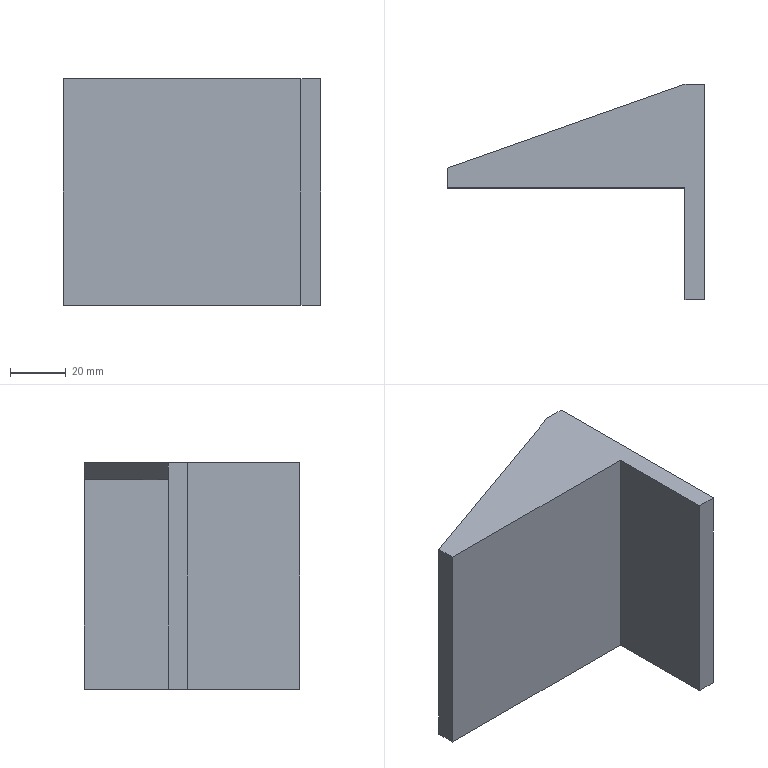Part | STEP file | Guide wheel mechanism revised.sldasm-Part-64 | 1 solid | 12 faces | box 92 x 77 x 81 mm | volume 99504 mm3 | plane 12
STEP:
#1=CARTESIAN_POINT('',(-42.5,0.,-40.5));
#2=VERTEX_POINT('',#1);
#3=CARTESIAN_POINT('',(-42.5,0.,40.5));
#4=VERTEX_POINT('',#3);
#5=CARTESIAN_POINT('',(-42.5,0.,40.5));
#6=DIRECTION('',(0.,0.,1.));
#7=VECTOR('',#6,1000.);
#8=LINE('',#5,#7);
#9=EDGE_CURVE('',#2,#4,#8,.T.);
#10=ORIENTED_EDGE('',*,*,#9,.T.);
#11=CARTESIAN_POINT('',(-42.5,7.,40.5));
#12=VERTEX_POINT('',#11);
#13=CARTESIAN_POINT('',(-42.5,7.,40.5));
#14=DIRECTION('',(0.,-1.,0.));
#15=VECTOR('',#14,1000.);
#16=LINE('',#13,#15);
#17=EDGE_CURVE('',#12,#4,#16,.T.);
#18=ORIENTED_EDGE('',*,*,#17,.F.);
#19=CARTESIAN_POINT('',(-42.5,7.,34.5));
#20=VERTEX_POINT('',#19);
#21=CARTESIAN_POINT('',(-42.5,7.,34.5));
#22=DIRECTION('',(0.,0.,1.));
#23=VECTOR('',#22,1000.);
#24=LINE('',#21,#23);
#25=EDGE_CURVE('',#20,#12,#24,.T.);
#26=ORIENTED_EDGE('',*,*,#25,.F.);
#27=CARTESIAN_POINT('',(-42.5,7.,-40.5));
#28=VERTEX_POINT('',#27);
#29=CARTESIAN_POINT('',(-42.5,7.,40.5));
#30=DIRECTION('',(0.,0.,1.));
#31=VECTOR('',#30,1000.);
#32=LINE('',#29,#31);
#33=EDGE_CURVE('',#28,#20,#32,.T.);
#34=ORIENTED_EDGE('',*,*,#33,.F.);
#35=CARTESIAN_POINT('',(-42.5,7.,-40.5));
#36=DIRECTION('',(0.,-1.,0.));
#37=VECTOR('',#36,1000.);
#38=LINE('',#35,#37);
#39=EDGE_CURVE('',#28,#2,#38,.T.);
#40=ORIENTED_EDGE('',*,*,#39,.T.);
#41=EDGE_LOOP('',(#10,#18,#26,#34,#40));
#42=FACE_OUTER_BOUND('',#41,.T.);
#43=CARTESIAN_POINT('',(-42.5,7.,40.5));
#44=DIRECTION('',(1.,0.,0.));
#45=DIRECTION('',(0.,0.,-1.));
#46=AXIS2_PLACEMENT_3D('',#43,#44,#45);
#47=PLANE('',#46);
#48=ADVANCED_FACE('',(#42),#47,.F.);
#49=CARTESIAN_POINT('',(42.5,37.,40.5));
#50=VERTEX_POINT('',#49);
#51=CARTESIAN_POINT('',(-42.5,7.,40.5));
#52=DIRECTION('',(0.943,0.3328,0.));
#53=VECTOR('',#52,1000.);
#54=LINE('',#51,#53);
#55=EDGE_CURVE('',#12,#50,#54,.T.);
#56=ORIENTED_EDGE('',*,*,#55,.F.);
#57=ORIENTED_EDGE('',*,*,#17,.T.);
#58=CARTESIAN_POINT('',(42.5,0.,40.5));
#59=VERTEX_POINT('',#58);
#60=CARTESIAN_POINT('',(42.5,0.,40.5));
#61=DIRECTION('',(1.,0.,0.));
#62=VECTOR('',#61,1000.);
#63=LINE('',#60,#62);
#64=EDGE_CURVE('',#4,#59,#63,.T.);
#65=ORIENTED_EDGE('',*,*,#64,.T.);
#66=CARTESIAN_POINT('',(42.5,-40.,40.5));
#67=VERTEX_POINT('',#66);
#68=CARTESIAN_POINT('',(42.5,37.,40.5));
#69=DIRECTION('',(0.,-1.,0.));
#70=VECTOR('',#69,1000.);
#71=LINE('',#68,#70);
#72=EDGE_CURVE('',#59,#67,#71,.T.);
#73=ORIENTED_EDGE('',*,*,#72,.T.);
#74=CARTESIAN_POINT('',(49.5,-40.,40.5));
#75=VERTEX_POINT('',#74);
#76=CARTESIAN_POINT('',(49.5,-40.,40.5));
#77=DIRECTION('',(-1.,0.,0.));
#78=VECTOR('',#77,1000.);
#79=LINE('',#76,#78);
#80=EDGE_CURVE('',#75,#67,#79,.T.);
#81=ORIENTED_EDGE('',*,*,#80,.F.);
#82=CARTESIAN_POINT('',(49.5,37.,40.5));
#83=VERTEX_POINT('',#82);
#84=CARTESIAN_POINT('',(49.5,37.,40.5));
#85=DIRECTION('',(0.,-1.,0.));
#86=VECTOR('',#85,1000.);
#87=LINE('',#84,#86);
#88=EDGE_CURVE('',#83,#75,#87,.T.);
#89=ORIENTED_EDGE('',*,*,#88,.F.);
#90=CARTESIAN_POINT('',(49.5,37.,40.5));
#91=DIRECTION('',(-1.,0.,0.));
#92=VECTOR('',#91,1000.);
#93=LINE('',#90,#92);
#94=EDGE_CURVE('',#83,#50,#93,.T.);
#95=ORIENTED_EDGE('',*,*,#94,.T.);
#96=EDGE_LOOP('',(#56,#57,#65,#73,#81,#89,#95));
#97=FACE_OUTER_BOUND('',#96,.T.);
#98=CARTESIAN_POINT('',(42.5,7.,40.5));
#99=DIRECTION('',(0.,0.,-1.));
#100=DIRECTION('',(-1.,0.,0.));
#101=AXIS2_PLACEMENT_3D('',#98,#99,#100);
#102=PLANE('',#101);
#103=ADVANCED_FACE('',(#97),#102,.F.);
#104=CARTESIAN_POINT('',(42.5,0.,-40.5));
#105=VERTEX_POINT('',#104);
#106=CARTESIAN_POINT('',(42.5,0.,-40.5));
#107=DIRECTION('',(-1.,0.,0.));
#108=VECTOR('',#107,1000.);
#109=LINE('',#106,#108);
#110=EDGE_CURVE('',#105,#2,#109,.T.);
#111=ORIENTED_EDGE('',*,*,#110,.T.);
#112=ORIENTED_EDGE('',*,*,#39,.F.);
#113=CARTESIAN_POINT('',(42.5,7.,-40.5));
#114=VERTEX_POINT('',#113);
#115=CARTESIAN_POINT('',(42.5,7.,-40.5));
#116=DIRECTION('',(-1.,0.,0.));
#117=VECTOR('',#116,1000.);
#118=LINE('',#115,#117);
#119=EDGE_CURVE('',#114,#28,#118,.T.);
#120=ORIENTED_EDGE('',*,*,#119,.F.);
#121=CARTESIAN_POINT('',(42.5,37.,-40.5));
#122=VERTEX_POINT('',#121);
#123=CARTESIAN_POINT('',(42.5,37.,-40.5));
#124=DIRECTION('',(0.,-1.,0.));
#125=VECTOR('',#124,1000.);
#126=LINE('',#123,#125);
#127=EDGE_CURVE('',#122,#114,#126,.T.);
#128=ORIENTED_EDGE('',*,*,#127,.F.);
#129=CARTESIAN_POINT('',(49.5,37.,-40.5));
#130=VERTEX_POINT('',#129);
#131=CARTESIAN_POINT('',(49.5,37.,-40.5));
#132=DIRECTION('',(-1.,0.,0.));
#133=VECTOR('',#132,1000.);
#134=LINE('',#131,#133);
#135=EDGE_CURVE('',#130,#122,#134,.T.);
#136=ORIENTED_EDGE('',*,*,#135,.F.);
#137=CARTESIAN_POINT('',(49.5,-40.,-40.5));
#138=VERTEX_POINT('',#137);
#139=CARTESIAN_POINT('',(49.5,37.,-40.5));
#140=DIRECTION('',(0.,-1.,0.));
#141=VECTOR('',#140,1000.);
#142=LINE('',#139,#141);
#143=EDGE_CURVE('',#130,#138,#142,.T.);
#144=ORIENTED_EDGE('',*,*,#143,.T.);
#145=CARTESIAN_POINT('',(42.5,-40.,-40.5));
#146=VERTEX_POINT('',#145);
#147=CARTESIAN_POINT('',(49.5,-40.,-40.5));
#148=DIRECTION('',(-1.,0.,0.));
#149=VECTOR('',#148,1000.);
#150=LINE('',#147,#149);
#151=EDGE_CURVE('',#138,#146,#150,.T.);
#152=ORIENTED_EDGE('',*,*,#151,.T.);
#153=CARTESIAN_POINT('',(42.5,37.,-40.5));
#154=DIRECTION('',(0.,-1.,0.));
#155=VECTOR('',#154,1000.);
#156=LINE('',#153,#155);
#157=EDGE_CURVE('',#105,#146,#156,.T.);
#158=ORIENTED_EDGE('',*,*,#157,.F.);
#159=EDGE_LOOP('',(#111,#112,#120,#128,#136,#144,#152,#158));
#160=FACE_OUTER_BOUND('',#159,.T.);
#161=CARTESIAN_POINT('',(42.5,7.,-40.5));
#162=DIRECTION('',(0.,0.,1.));
#163=DIRECTION('',(1.,0.,0.));
#164=AXIS2_PLACEMENT_3D('',#161,#162,#163);
#165=PLANE('',#164);
#166=ADVANCED_FACE('',(#160),#165,.F.);
#167=CARTESIAN_POINT('',(42.5,7.,34.5));
#168=VERTEX_POINT('',#167);
#169=CARTESIAN_POINT('',(42.5,7.,34.5));
#170=DIRECTION('',(-1.,0.,0.));
#171=VECTOR('',#170,1000.);
#172=LINE('',#169,#171);
#173=EDGE_CURVE('',#168,#20,#172,.T.);
#174=ORIENTED_EDGE('',*,*,#173,.F.);
#175=CARTESIAN_POINT('',(42.5,7.,40.5));
#176=DIRECTION('',(0.,0.,-1.));
#177=VECTOR('',#176,1000.);
#178=LINE('',#175,#177);
#179=EDGE_CURVE('',#168,#114,#178,.T.);
#180=ORIENTED_EDGE('',*,*,#179,.T.);
#181=ORIENTED_EDGE('',*,*,#119,.T.);
#182=ORIENTED_EDGE('',*,*,#33,.T.);
#183=EDGE_LOOP('',(#174,#180,#181,#182));
#184=FACE_OUTER_BOUND('',#183,.T.);
#185=CARTESIAN_POINT('',(0.,7.,0.));
#186=DIRECTION('',(0.,1.,0.));
#187=DIRECTION('',(0.,0.,1.));
#188=AXIS2_PLACEMENT_3D('',#185,#186,#187);
#189=PLANE('',#188);
#190=ADVANCED_FACE('',(#184),#189,.T.);
#191=ORIENTED_EDGE('',*,*,#9,.F.);
#192=ORIENTED_EDGE('',*,*,#110,.F.);
#193=CARTESIAN_POINT('',(42.5,0.,40.5));
#194=DIRECTION('',(0.,0.,-1.));
#195=VECTOR('',#194,1000.);
#196=LINE('',#193,#195);
#197=EDGE_CURVE('',#59,#105,#196,.T.);
#198=ORIENTED_EDGE('',*,*,#197,.F.);
#199=ORIENTED_EDGE('',*,*,#64,.F.);
#200=EDGE_LOOP('',(#191,#192,#198,#199));
#201=FACE_OUTER_BOUND('',#200,.T.);
#202=CARTESIAN_POINT('',(0.,0.,0.));
#203=DIRECTION('',(0.,1.,0.));
#204=DIRECTION('',(0.,0.,1.));
#205=AXIS2_PLACEMENT_3D('',#202,#203,#204);
#206=PLANE('',#205);
#207=ADVANCED_FACE('',(#201),#206,.F.);
#208=ORIENTED_EDGE('',*,*,#55,.T.);
#209=CARTESIAN_POINT('',(42.5,37.,34.5));
#210=VERTEX_POINT('',#209);
#211=CARTESIAN_POINT('',(42.5,37.,40.5));
#212=DIRECTION('',(0.,0.,-1.));
#213=VECTOR('',#212,1000.);
#214=LINE('',#211,#213);
#215=EDGE_CURVE('',#50,#210,#214,.T.);
#216=ORIENTED_EDGE('',*,*,#215,.T.);
#217=CARTESIAN_POINT('',(-42.5,7.,34.5));
#218=DIRECTION('',(0.943,0.3328,0.));
#219=VECTOR('',#218,1000.);
#220=LINE('',#217,#219);
#221=EDGE_CURVE('',#20,#210,#220,.T.);
#222=ORIENTED_EDGE('',*,*,#221,.F.);
#223=ORIENTED_EDGE('',*,*,#25,.T.);
#224=EDGE_LOOP('',(#208,#216,#222,#223));
#225=FACE_OUTER_BOUND('',#224,.T.);
#226=CARTESIAN_POINT('',(-42.5,7.,34.5));
#227=DIRECTION('',(-0.3328,0.943,0.));
#228=DIRECTION('',(-0.943,-0.3328,0.));
#229=AXIS2_PLACEMENT_3D('',#226,#227,#228);
#230=PLANE('',#229);
#231=ADVANCED_FACE('',(#225),#230,.T.);
#232=ORIENTED_EDGE('',*,*,#221,.T.);
#233=CARTESIAN_POINT('',(42.5,37.,34.5));
#234=DIRECTION('',(0.,-1.,0.));
#235=VECTOR('',#234,1000.);
#236=LINE('',#233,#235);
#237=EDGE_CURVE('',#210,#168,#236,.T.);
#238=ORIENTED_EDGE('',*,*,#237,.T.);
#239=ORIENTED_EDGE('',*,*,#173,.T.);
#240=EDGE_LOOP('',(#232,#238,#239));
#241=FACE_OUTER_BOUND('',#240,.T.);
#242=CARTESIAN_POINT('',(0.,0.,34.5));
#243=DIRECTION('',(0.,0.,1.));
#244=DIRECTION('',(0.,1.,0.));
#245=AXIS2_PLACEMENT_3D('',#242,#243,#244);
#246=PLANE('',#245);
#247=ADVANCED_FACE('',(#241),#246,.F.);
#248=ORIENTED_EDGE('',*,*,#197,.T.);
#249=ORIENTED_EDGE('',*,*,#157,.T.);
#250=CARTESIAN_POINT('',(42.5,-40.,40.5));
#251=DIRECTION('',(0.,0.,-1.));
#252=VECTOR('',#251,1000.);
#253=LINE('',#250,#252);
#254=EDGE_CURVE('',#67,#146,#253,.T.);
#255=ORIENTED_EDGE('',*,*,#254,.F.);
#256=ORIENTED_EDGE('',*,*,#72,.F.);
#257=EDGE_LOOP('',(#248,#249,#255,#256));
#258=FACE_OUTER_BOUND('',#257,.T.);
#259=CARTESIAN_POINT('',(42.5,0.,0.));
#260=DIRECTION('',(-1.,0.,0.));
#261=DIRECTION('',(0.,0.,1.));
#262=AXIS2_PLACEMENT_3D('',#259,#260,#261);
#263=PLANE('',#262);
#264=ADVANCED_FACE('',(#258),#263,.T.);
#265=ORIENTED_EDGE('',*,*,#215,.F.);
#266=ORIENTED_EDGE('',*,*,#94,.F.);
#267=CARTESIAN_POINT('',(49.5,37.,40.5));
#268=DIRECTION('',(0.,0.,-1.));
#269=VECTOR('',#268,1000.);
#270=LINE('',#267,#269);
#271=EDGE_CURVE('',#83,#130,#270,.T.);
#272=ORIENTED_EDGE('',*,*,#271,.T.);
#273=ORIENTED_EDGE('',*,*,#135,.T.);
#274=CARTESIAN_POINT('',(42.5,37.,40.5));
#275=DIRECTION('',(0.,0.,-1.));
#276=VECTOR('',#275,1000.);
#277=LINE('',#274,#276);
#278=EDGE_CURVE('',#210,#122,#277,.T.);
#279=ORIENTED_EDGE('',*,*,#278,.F.);
#280=EDGE_LOOP('',(#265,#266,#272,#273,#279));
#281=FACE_OUTER_BOUND('',#280,.T.);
#282=CARTESIAN_POINT('',(49.5,37.,40.5));
#283=DIRECTION('',(0.,1.,0.));
#284=DIRECTION('',(0.,0.,1.));
#285=AXIS2_PLACEMENT_3D('',#282,#283,#284);
#286=PLANE('',#285);
#287=ADVANCED_FACE('',(#281),#286,.T.);
#288=ORIENTED_EDGE('',*,*,#254,.T.);
#289=ORIENTED_EDGE('',*,*,#151,.F.);
#290=CARTESIAN_POINT('',(49.5,-40.,40.5));
#291=DIRECTION('',(0.,0.,-1.));
#292=VECTOR('',#291,1000.);
#293=LINE('',#290,#292);
#294=EDGE_CURVE('',#75,#138,#293,.T.);
#295=ORIENTED_EDGE('',*,*,#294,.F.);
#296=ORIENTED_EDGE('',*,*,#80,.T.);
#297=EDGE_LOOP('',(#288,#289,#295,#296));
#298=FACE_OUTER_BOUND('',#297,.T.);
#299=CARTESIAN_POINT('',(49.5,-40.,40.5));
#300=DIRECTION('',(0.,1.,0.));
#301=DIRECTION('',(0.,0.,1.));
#302=AXIS2_PLACEMENT_3D('',#299,#300,#301);
#303=PLANE('',#302);
#304=ADVANCED_FACE('',(#298),#303,.F.);
#305=ORIENTED_EDGE('',*,*,#271,.F.);
#306=ORIENTED_EDGE('',*,*,#88,.T.);
#307=ORIENTED_EDGE('',*,*,#294,.T.);
#308=ORIENTED_EDGE('',*,*,#143,.F.);
#309=EDGE_LOOP('',(#305,#306,#307,#308));
#310=FACE_OUTER_BOUND('',#309,.T.);
#311=CARTESIAN_POINT('',(49.5,0.,0.));
#312=DIRECTION('',(-1.,0.,0.));
#313=DIRECTION('',(0.,0.,1.));
#314=AXIS2_PLACEMENT_3D('',#311,#312,#313);
#315=PLANE('',#314);
#316=ADVANCED_FACE('',(#310),#315,.F.);
#317=ORIENTED_EDGE('',*,*,#127,.T.);
#318=ORIENTED_EDGE('',*,*,#179,.F.);
#319=ORIENTED_EDGE('',*,*,#237,.F.);
#320=ORIENTED_EDGE('',*,*,#278,.T.);
#321=EDGE_LOOP('',(#317,#318,#319,#320));
#322=FACE_OUTER_BOUND('',#321,.T.);
#323=CARTESIAN_POINT('',(42.5,0.,0.));
#324=DIRECTION('',(-1.,0.,0.));
#325=DIRECTION('',(0.,0.,1.));
#326=AXIS2_PLACEMENT_3D('',#323,#324,#325);
#327=PLANE('',#326);
#328=ADVANCED_FACE('',(#322),#327,.T.);
#329=CLOSED_SHELL('',(#48,#103,#166,#190,#207,#231,#247,#264,#287,#304,#316,#328));
#330=MANIFOLD_SOLID_BREP('',#329);
#331=CARTESIAN_POINT('',(0.,0.,0.));
#332=DIRECTION('',(0.,0.,1.));
#333=DIRECTION('',(1.,0.,0.));
#334=AXIS2_PLACEMENT_3D('',#331,#332,#333);
#335=(LENGTH_UNIT()NAMED_UNIT(*)SI_UNIT(.MILLI.,.METRE.));
#336=UNCERTAINTY_MEASURE_WITH_UNIT(LENGTH_MEASURE(0.00001),#335,'','');
#337=(NAMED_UNIT(*)PLANE_ANGLE_UNIT()SI_UNIT($,.RADIAN.));
#338=(NAMED_UNIT(*)SI_UNIT($,.STERADIAN.)SOLID_ANGLE_UNIT());
#339=(GEOMETRIC_REPRESENTATION_CONTEXT(3)GLOBAL_UNCERTAINTY_ASSIGNED_CONTEXT((#336))GLOBAL_UNIT_ASSIGNED_CONTEXT((#335,#337,#338))REPRESENTATION_CONTEXT('',''));
#340=ADVANCED_BREP_SHAPE_REPRESENTATION('',(#330,#334),#339);